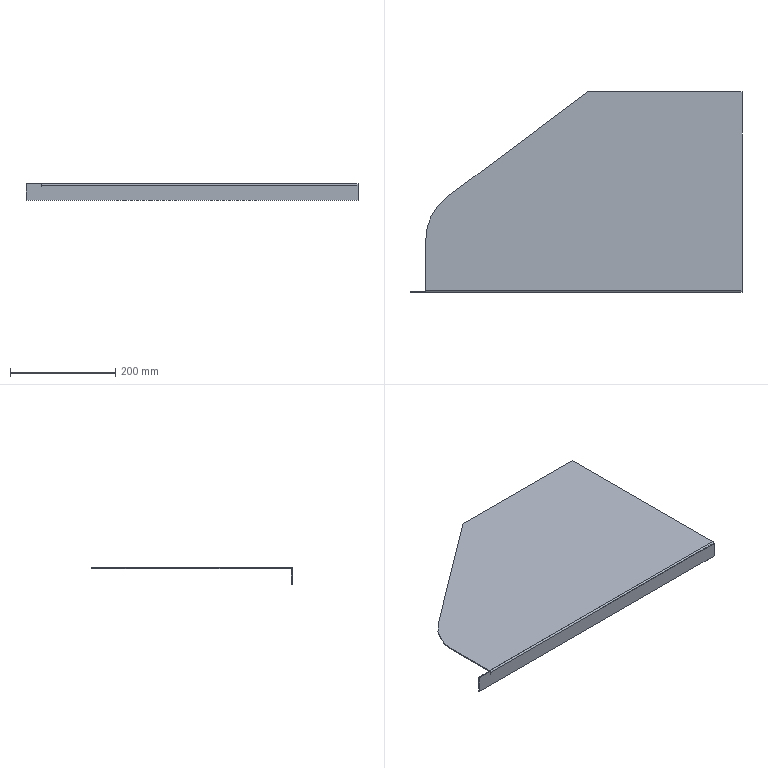Part | SolidWorks | features ICE 5, Split 4, DeleteBody 3, Extrusion 1, FlatPattern 1, SheetMetal 1, Shell 1, SolidToSheetMetal 1 | 1 solid | 20 faces | box 630 x 380 x 32 mm | volume 421618 mm3 | plane 17 | cylinder 3 | commonest cylinder face diameters 2 x1 6 x1 200 x1
STEP:
#1=CARTESIAN_POINT('',(-1100.,3.,-298.));
#2=VERTEX_POINT('',#1);
#3=CARTESIAN_POINT('',(-1100.,3.,-300.));
#4=VERTEX_POINT('',#3);
#5=CARTESIAN_POINT('',(-1100.,3.,-300.));
#6=DIRECTION('',(0.,0.,-1.));
#7=VECTOR('',#6,1000.);
#8=LINE('',#5,#7);
#9=EDGE_CURVE('',#2,#4,#8,.T.);
#10=ORIENTED_EDGE('',*,*,#9,.F.);
#11=CARTESIAN_POINT('',(-1100.,100.,-298.));
#12=VERTEX_POINT('',#11);
#13=CARTESIAN_POINT('',(-1100.,100.,-298.));
#14=DIRECTION('',(0.,1.,0.));
#15=VECTOR('',#14,1000.);
#16=LINE('',#13,#15);
#17=EDGE_CURVE('',#2,#12,#16,.T.);
#18=ORIENTED_EDGE('',*,*,#17,.T.);
#19=CARTESIAN_POINT('',(-1100.,100.,-300.));
#20=VERTEX_POINT('',#19);
#21=CARTESIAN_POINT('',(-1100.,100.,-300.));
#22=DIRECTION('',(0.,0.,-1.));
#23=VECTOR('',#22,1000.);
#24=LINE('',#21,#23);
#25=EDGE_CURVE('',#12,#20,#24,.T.);
#26=ORIENTED_EDGE('',*,*,#25,.T.);
#27=CARTESIAN_POINT('',(-1100.,100.,-300.));
#28=DIRECTION('',(0.,1.,0.));
#29=VECTOR('',#28,1000.);
#30=LINE('',#27,#29);
#31=EDGE_CURVE('',#4,#20,#30,.T.);
#32=ORIENTED_EDGE('',*,*,#31,.F.);
#33=EDGE_LOOP('',(#10,#18,#26,#32));
#34=FACE_OUTER_BOUND('',#33,.T.);
#35=CARTESIAN_POINT('',(-1100.,100.,-300.));
#36=DIRECTION('',(-1.,0.,0.));
#37=DIRECTION('',(0.,1.,0.));
#38=AXIS2_PLACEMENT_3D('',#35,#36,#37);
#39=PLANE('',#38);
#40=ADVANCED_FACE('',(#34),#39,.T.);
#41=ORIENTED_EDGE('',*,*,#25,.F.);
#42=CARTESIAN_POINT('',(-1060.,180.,-298.));
#43=VERTEX_POINT('',#42);
#44=CARTESIAN_POINT('',(-1000.,100.,-298.));
#45=DIRECTION('',(0.,0.,-1.));
#46=DIRECTION('',(-1.,0.,0.));
#47=AXIS2_PLACEMENT_3D('',#44,#45,#46);
#48=CIRCLE('',#47,100.);
#49=EDGE_CURVE('',#12,#43,#48,.T.);
#50=ORIENTED_EDGE('',*,*,#49,.T.);
#51=CARTESIAN_POINT('',(-1060.,180.,-300.));
#52=VERTEX_POINT('',#51);
#53=CARTESIAN_POINT('',(-1060.,180.,-300.));
#54=DIRECTION('',(0.,0.,-1.));
#55=VECTOR('',#54,1000.);
#56=LINE('',#53,#55);
#57=EDGE_CURVE('',#43,#52,#56,.T.);
#58=ORIENTED_EDGE('',*,*,#57,.T.);
#59=CARTESIAN_POINT('',(-1000.,100.,-300.));
#60=DIRECTION('',(0.,0.,-1.));
#61=DIRECTION('',(-1.,0.,0.));
#62=AXIS2_PLACEMENT_3D('',#59,#60,#61);
#63=CIRCLE('',#62,100.);
#64=EDGE_CURVE('',#20,#52,#63,.T.);
#65=ORIENTED_EDGE('',*,*,#64,.F.);
#66=EDGE_LOOP('',(#41,#50,#58,#65));
#67=FACE_OUTER_BOUND('',#66,.T.);
#68=CARTESIAN_POINT('',(-1000.,100.,-300.));
#69=DIRECTION('',(0.,0.,-1.));
#70=DIRECTION('',(-1.,0.,0.));
#71=AXIS2_PLACEMENT_3D('',#68,#69,#70);
#72=CYLINDRICAL_SURFACE('',#71,100.);
#73=ADVANCED_FACE('',(#67),#72,.T.);
#74=ORIENTED_EDGE('',*,*,#57,.F.);
#75=CARTESIAN_POINT('',(-793.333,380.,-298.));
#76=VERTEX_POINT('',#75);
#77=CARTESIAN_POINT('',(-793.333,380.,-298.));
#78=DIRECTION('',(0.8,0.6,0.));
#79=VECTOR('',#78,1000.);
#80=LINE('',#77,#79);
#81=EDGE_CURVE('',#43,#76,#80,.T.);
#82=ORIENTED_EDGE('',*,*,#81,.T.);
#83=CARTESIAN_POINT('',(-793.333,380.,-300.));
#84=VERTEX_POINT('',#83);
#85=CARTESIAN_POINT('',(-793.333,380.,-300.));
#86=DIRECTION('',(0.,0.,-1.));
#87=VECTOR('',#86,1000.);
#88=LINE('',#85,#87);
#89=EDGE_CURVE('',#76,#84,#88,.T.);
#90=ORIENTED_EDGE('',*,*,#89,.T.);
#91=CARTESIAN_POINT('',(-793.333,380.,-300.));
#92=DIRECTION('',(0.8,0.6,0.));
#93=VECTOR('',#92,1000.);
#94=LINE('',#91,#93);
#95=EDGE_CURVE('',#52,#84,#94,.T.);
#96=ORIENTED_EDGE('',*,*,#95,.F.);
#97=EDGE_LOOP('',(#74,#82,#90,#96));
#98=FACE_OUTER_BOUND('',#97,.T.);
#99=CARTESIAN_POINT('',(-793.333,380.,-300.));
#100=DIRECTION('',(-0.6,0.8,0.));
#101=DIRECTION('',(0.8,0.6,0.));
#102=AXIS2_PLACEMENT_3D('',#99,#100,#101);
#103=PLANE('',#102);
#104=ADVANCED_FACE('',(#98),#103,.T.);
#105=ORIENTED_EDGE('',*,*,#89,.F.);
#106=CARTESIAN_POINT('',(-500.,380.,-298.));
#107=VERTEX_POINT('',#106);
#108=CARTESIAN_POINT('',(-1000.,380.,-298.));
#109=DIRECTION('',(1.,0.,0.));
#110=VECTOR('',#109,1000.);
#111=LINE('',#108,#110);
#112=EDGE_CURVE('',#76,#107,#111,.T.);
#113=ORIENTED_EDGE('',*,*,#112,.T.);
#114=CARTESIAN_POINT('',(-500.,380.,-300.));
#115=VERTEX_POINT('',#114);
#116=CARTESIAN_POINT('',(-500.,380.,-300.));
#117=DIRECTION('',(0.,0.,-1.));
#118=VECTOR('',#117,1000.);
#119=LINE('',#116,#118);
#120=EDGE_CURVE('',#107,#115,#119,.T.);
#121=ORIENTED_EDGE('',*,*,#120,.T.);
#122=CARTESIAN_POINT('',(-793.333,380.,-300.));
#123=DIRECTION('',(1.,0.,0.));
#124=VECTOR('',#123,1000.);
#125=LINE('',#122,#124);
#126=EDGE_CURVE('',#84,#115,#125,.T.);
#127=ORIENTED_EDGE('',*,*,#126,.F.);
#128=EDGE_LOOP('',(#105,#113,#121,#127));
#129=FACE_OUTER_BOUND('',#128,.T.);
#130=CARTESIAN_POINT('',(-793.333,380.,-300.));
#131=DIRECTION('',(0.,1.,0.));
#132=DIRECTION('',(1.,0.,0.));
#133=AXIS2_PLACEMENT_3D('',#130,#131,#132);
#134=PLANE('',#133);
#135=ADVANCED_FACE('',(#129),#134,.T.);
#136=ORIENTED_EDGE('',*,*,#120,.F.);
#137=CARTESIAN_POINT('',(-500.,3.,-298.));
#138=VERTEX_POINT('',#137);
#139=CARTESIAN_POINT('',(-500.,100.,-298.));
#140=DIRECTION('',(0.,-1.,0.));
#141=VECTOR('',#140,1000.);
#142=LINE('',#139,#141);
#143=EDGE_CURVE('',#107,#138,#142,.T.);
#144=ORIENTED_EDGE('',*,*,#143,.T.);
#145=CARTESIAN_POINT('',(-500.,3.,-300.));
#146=VERTEX_POINT('',#145);
#147=CARTESIAN_POINT('',(-500.,3.,-300.));
#148=DIRECTION('',(0.,0.,-1.));
#149=VECTOR('',#148,1000.);
#150=LINE('',#147,#149);
#151=EDGE_CURVE('',#138,#146,#150,.T.);
#152=ORIENTED_EDGE('',*,*,#151,.T.);
#153=CARTESIAN_POINT('',(-500.,380.,-300.));
#154=DIRECTION('',(0.,-1.,0.));
#155=VECTOR('',#154,1000.);
#156=LINE('',#153,#155);
#157=EDGE_CURVE('',#115,#146,#156,.T.);
#158=ORIENTED_EDGE('',*,*,#157,.F.);
#159=EDGE_LOOP('',(#136,#144,#152,#158));
#160=FACE_OUTER_BOUND('',#159,.T.);
#161=CARTESIAN_POINT('',(-500.,380.,-300.));
#162=DIRECTION('',(1.,0.,0.));
#163=DIRECTION('',(0.,-1.,0.));
#164=AXIS2_PLACEMENT_3D('',#161,#162,#163);
#165=PLANE('',#164);
#166=ADVANCED_FACE('',(#160),#165,.T.);
#167=ORIENTED_EDGE('',*,*,#151,.F.);
#168=CARTESIAN_POINT('',(-500.,0.,-301.));
#169=VERTEX_POINT('',#168);
#170=CARTESIAN_POINT('',(-500.,3.,-301.));
#171=DIRECTION('',(1.,0.,0.));
#172=DIRECTION('',(0.,0.,-1.));
#173=AXIS2_PLACEMENT_3D('',#170,#171,#172);
#174=CIRCLE('',#173,3.);
#175=EDGE_CURVE('',#138,#169,#174,.T.);
#176=ORIENTED_EDGE('',*,*,#175,.T.);
#177=CARTESIAN_POINT('',(-500.,2.,-301.));
#178=VERTEX_POINT('',#177);
#179=CARTESIAN_POINT('',(-500.,2.,-301.));
#180=DIRECTION('',(0.,1.,0.));
#181=VECTOR('',#180,1000.);
#182=LINE('',#179,#181);
#183=EDGE_CURVE('',#169,#178,#182,.T.);
#184=ORIENTED_EDGE('',*,*,#183,.T.);
#185=CARTESIAN_POINT('',(-500.,3.,-301.));
#186=DIRECTION('',(1.,0.,0.));
#187=DIRECTION('',(0.,0.,1.));
#188=AXIS2_PLACEMENT_3D('',#185,#186,#187);
#189=CIRCLE('',#188,1.);
#190=EDGE_CURVE('',#146,#178,#189,.T.);
#191=ORIENTED_EDGE('',*,*,#190,.F.);
#192=EDGE_LOOP('',(#167,#176,#184,#191));
#193=FACE_OUTER_BOUND('',#192,.T.);
#194=CARTESIAN_POINT('',(-500.,3.,-301.));
#195=DIRECTION('',(1.,0.,0.));
#196=DIRECTION('',(0.,0.,-1.));
#197=AXIS2_PLACEMENT_3D('',#194,#195,#196);
#198=PLANE('',#197);
#199=ADVANCED_FACE('',(#193),#198,.T.);
#200=ORIENTED_EDGE('',*,*,#183,.F.);
#201=CARTESIAN_POINT('',(-500.,0.,-330.));
#202=VERTEX_POINT('',#201);
#203=CARTESIAN_POINT('',(-500.,0.,0.));
#204=DIRECTION('',(0.,0.,-1.));
#205=VECTOR('',#204,1000.);
#206=LINE('',#203,#205);
#207=EDGE_CURVE('',#169,#202,#206,.T.);
#208=ORIENTED_EDGE('',*,*,#207,.T.);
#209=CARTESIAN_POINT('',(-500.,2.,-330.));
#210=VERTEX_POINT('',#209);
#211=CARTESIAN_POINT('',(-500.,2.,-330.));
#212=DIRECTION('',(0.,1.,0.));
#213=VECTOR('',#212,1000.);
#214=LINE('',#211,#213);
#215=EDGE_CURVE('',#202,#210,#214,.T.);
#216=ORIENTED_EDGE('',*,*,#215,.T.);
#217=CARTESIAN_POINT('',(-500.,2.,0.));
#218=DIRECTION('',(0.,0.,-1.));
#219=VECTOR('',#218,1000.);
#220=LINE('',#217,#219);
#221=EDGE_CURVE('',#178,#210,#220,.T.);
#222=ORIENTED_EDGE('',*,*,#221,.F.);
#223=EDGE_LOOP('',(#200,#208,#216,#222));
#224=FACE_OUTER_BOUND('',#223,.T.);
#225=CARTESIAN_POINT('',(-500.,2.,0.));
#226=DIRECTION('',(1.,0.,0.));
#227=DIRECTION('',(0.,0.,-1.));
#228=AXIS2_PLACEMENT_3D('',#225,#226,#227);
#229=PLANE('',#228);
#230=ADVANCED_FACE('',(#224),#229,.T.);
#231=ORIENTED_EDGE('',*,*,#215,.F.);
#232=CARTESIAN_POINT('',(-1130.,0.,-330.));
#233=VERTEX_POINT('',#232);
#234=CARTESIAN_POINT('',(0.,0.,-330.));
#235=DIRECTION('',(1.,0.,0.));
#236=VECTOR('',#235,1000.);
#237=LINE('',#234,#236);
#238=EDGE_CURVE('',#233,#202,#237,.T.);
#239=ORIENTED_EDGE('',*,*,#238,.F.);
#240=CARTESIAN_POINT('',(-1130.,2.,-330.));
#241=VERTEX_POINT('',#240);
#242=CARTESIAN_POINT('',(-1130.,2.,-330.));
#243=DIRECTION('',(0.,1.,0.));
#244=VECTOR('',#243,1000.);
#245=LINE('',#242,#244);
#246=EDGE_CURVE('',#233,#241,#245,.T.);
#247=ORIENTED_EDGE('',*,*,#246,.T.);
#248=CARTESIAN_POINT('',(-1130.,2.,-330.));
#249=DIRECTION('',(1.,0.,0.));
#250=VECTOR('',#249,1000.);
#251=LINE('',#248,#250);
#252=EDGE_CURVE('',#241,#210,#251,.T.);
#253=ORIENTED_EDGE('',*,*,#252,.T.);
#254=EDGE_LOOP('',(#231,#239,#247,#253));
#255=FACE_OUTER_BOUND('',#254,.T.);
#256=CARTESIAN_POINT('',(-1130.,2.,-330.));
#257=DIRECTION('',(0.,0.,1.));
#258=DIRECTION('',(1.,0.,0.));
#259=AXIS2_PLACEMENT_3D('',#256,#257,#258);
#260=PLANE('',#259);
#261=ADVANCED_FACE('',(#255),#260,.F.);
#262=ORIENTED_EDGE('',*,*,#246,.F.);
#263=CARTESIAN_POINT('',(-1130.,0.,-298.));
#264=VERTEX_POINT('',#263);
#265=CARTESIAN_POINT('',(-1130.,0.,0.));
#266=DIRECTION('',(0.,0.,-1.));
#267=VECTOR('',#266,1000.);
#268=LINE('',#265,#267);
#269=EDGE_CURVE('',#264,#233,#268,.T.);
#270=ORIENTED_EDGE('',*,*,#269,.F.);
#271=CARTESIAN_POINT('',(-1130.,2.,-298.));
#272=VERTEX_POINT('',#271);
#273=CARTESIAN_POINT('',(-1130.,2.,-298.));
#274=DIRECTION('',(0.,1.,0.));
#275=VECTOR('',#274,1000.);
#276=LINE('',#273,#275);
#277=EDGE_CURVE('',#264,#272,#276,.T.);
#278=ORIENTED_EDGE('',*,*,#277,.T.);
#279=CARTESIAN_POINT('',(-1130.,2.,0.));
#280=DIRECTION('',(0.,0.,-1.));
#281=VECTOR('',#280,1000.);
#282=LINE('',#279,#281);
#283=EDGE_CURVE('',#272,#241,#282,.T.);
#284=ORIENTED_EDGE('',*,*,#283,.T.);
#285=EDGE_LOOP('',(#262,#270,#278,#284));
#286=FACE_OUTER_BOUND('',#285,.T.);
#287=CARTESIAN_POINT('',(-1130.,2.,0.));
#288=DIRECTION('',(1.,0.,0.));
#289=DIRECTION('',(0.,0.,-1.));
#290=AXIS2_PLACEMENT_3D('',#287,#288,#289);
#291=PLANE('',#290);
#292=ADVANCED_FACE('',(#286),#291,.F.);
#293=ORIENTED_EDGE('',*,*,#277,.F.);
#294=CARTESIAN_POINT('',(-1101.,0.,-298.));
#295=VERTEX_POINT('',#294);
#296=CARTESIAN_POINT('',(0.,0.,-298.));
#297=DIRECTION('',(1.,0.,0.));
#298=VECTOR('',#297,1000.);
#299=LINE('',#296,#298);
#300=EDGE_CURVE('',#264,#295,#299,.T.);
#301=ORIENTED_EDGE('',*,*,#300,.T.);
#302=CARTESIAN_POINT('',(-1101.,2.,-298.));
#303=VERTEX_POINT('',#302);
#304=CARTESIAN_POINT('',(-1101.,2.,-298.));
#305=DIRECTION('',(0.,1.,0.));
#306=VECTOR('',#305,1000.);
#307=LINE('',#304,#306);
#308=EDGE_CURVE('',#295,#303,#307,.T.);
#309=ORIENTED_EDGE('',*,*,#308,.T.);
#310=CARTESIAN_POINT('',(0.,2.,-298.));
#311=DIRECTION('',(1.,0.,0.));
#312=VECTOR('',#311,1000.);
#313=LINE('',#310,#312);
#314=EDGE_CURVE('',#272,#303,#313,.T.);
#315=ORIENTED_EDGE('',*,*,#314,.F.);
#316=EDGE_LOOP('',(#293,#301,#309,#315));
#317=FACE_OUTER_BOUND('',#316,.T.);
#318=CARTESIAN_POINT('',(0.,2.,-298.));
#319=DIRECTION('',(0.,0.,1.));
#320=DIRECTION('',(1.,0.,0.));
#321=AXIS2_PLACEMENT_3D('',#318,#319,#320);
#322=PLANE('',#321);
#323=ADVANCED_FACE('',(#317),#322,.T.);
#324=ORIENTED_EDGE('',*,*,#308,.F.);
#325=CARTESIAN_POINT('',(-1101.,0.,-304.));
#326=VERTEX_POINT('',#325);
#327=CARTESIAN_POINT('',(-1101.,0.,0.));
#328=DIRECTION('',(0.,0.,1.));
#329=VECTOR('',#328,1000.);
#330=LINE('',#327,#329);
#331=EDGE_CURVE('',#326,#295,#330,.T.);
#332=ORIENTED_EDGE('',*,*,#331,.F.);
#333=CARTESIAN_POINT('',(-1101.,2.,-304.));
#334=VERTEX_POINT('',#333);
#335=CARTESIAN_POINT('',(-1101.,2.,-304.));
#336=DIRECTION('',(0.,1.,0.));
#337=VECTOR('',#336,1000.);
#338=LINE('',#335,#337);
#339=EDGE_CURVE('',#326,#334,#338,.T.);
#340=ORIENTED_EDGE('',*,*,#339,.T.);
#341=CARTESIAN_POINT('',(-1101.,2.,0.));
#342=DIRECTION('',(0.,0.,1.));
#343=VECTOR('',#342,1000.);
#344=LINE('',#341,#343);
#345=EDGE_CURVE('',#334,#303,#344,.T.);
#346=ORIENTED_EDGE('',*,*,#345,.T.);
#347=EDGE_LOOP('',(#324,#332,#340,#346));
#348=FACE_OUTER_BOUND('',#347,.T.);
#349=CARTESIAN_POINT('',(-1101.,2.,0.));
#350=DIRECTION('',(-1.,0.,0.));
#351=DIRECTION('',(0.,0.,1.));
#352=AXIS2_PLACEMENT_3D('',#349,#350,#351);
#353=PLANE('',#352);
#354=ADVANCED_FACE('',(#348),#353,.F.);
#355=ORIENTED_EDGE('',*,*,#339,.F.);
#356=CARTESIAN_POINT('',(-1100.,0.,-304.));
#357=VERTEX_POINT('',#356);
#358=CARTESIAN_POINT('',(0.,0.,-304.));
#359=DIRECTION('',(-1.,0.,0.));
#360=VECTOR('',#359,1000.);
#361=LINE('',#358,#360);
#362=EDGE_CURVE('',#357,#326,#361,.T.);
#363=ORIENTED_EDGE('',*,*,#362,.F.);
#364=CARTESIAN_POINT('',(-1100.,2.,-304.));
#365=VERTEX_POINT('',#364);
#366=CARTESIAN_POINT('',(-1100.,2.,-304.));
#367=DIRECTION('',(0.,1.,0.));
#368=VECTOR('',#367,1000.);
#369=LINE('',#366,#368);
#370=EDGE_CURVE('',#357,#365,#369,.T.);
#371=ORIENTED_EDGE('',*,*,#370,.T.);
#372=CARTESIAN_POINT('',(0.,2.,-304.));
#373=DIRECTION('',(-1.,0.,0.));
#374=VECTOR('',#373,1000.);
#375=LINE('',#372,#374);
#376=EDGE_CURVE('',#365,#334,#375,.T.);
#377=ORIENTED_EDGE('',*,*,#376,.T.);
#378=EDGE_LOOP('',(#355,#363,#371,#377));
#379=FACE_OUTER_BOUND('',#378,.T.);
#380=CARTESIAN_POINT('',(0.,2.,-304.));
#381=DIRECTION('',(0.,0.,-1.));
#382=DIRECTION('',(-1.,0.,0.));
#383=AXIS2_PLACEMENT_3D('',#380,#381,#382);
#384=PLANE('',#383);
#385=ADVANCED_FACE('',(#379),#384,.F.);
#386=ORIENTED_EDGE('',*,*,#370,.F.);
#387=CARTESIAN_POINT('',(-1100.,0.,-301.));
#388=VERTEX_POINT('',#387);
#389=CARTESIAN_POINT('',(-1100.,0.,0.));
#390=DIRECTION('',(0.,0.,-1.));
#391=VECTOR('',#390,1000.);
#392=LINE('',#389,#391);
#393=EDGE_CURVE('',#388,#357,#392,.T.);
#394=ORIENTED_EDGE('',*,*,#393,.F.);
#395=CARTESIAN_POINT('',(-1100.,2.,-301.));
#396=VERTEX_POINT('',#395);
#397=CARTESIAN_POINT('',(-1100.,2.,-301.));
#398=DIRECTION('',(0.,1.,0.));
#399=VECTOR('',#398,1000.);
#400=LINE('',#397,#399);
#401=EDGE_CURVE('',#388,#396,#400,.T.);
#402=ORIENTED_EDGE('',*,*,#401,.T.);
#403=CARTESIAN_POINT('',(-1100.,2.,0.));
#404=DIRECTION('',(0.,0.,-1.));
#405=VECTOR('',#404,1000.);
#406=LINE('',#403,#405);
#407=EDGE_CURVE('',#396,#365,#406,.T.);
#408=ORIENTED_EDGE('',*,*,#407,.T.);
#409=EDGE_LOOP('',(#386,#394,#402,#408));
#410=FACE_OUTER_BOUND('',#409,.T.);
#411=CARTESIAN_POINT('',(-1100.,2.,0.));
#412=DIRECTION('',(1.,0.,0.));
#413=DIRECTION('',(0.,0.,-1.));
#414=AXIS2_PLACEMENT_3D('',#411,#412,#413);
#415=PLANE('',#414);
#416=ADVANCED_FACE('',(#410),#415,.F.);
#417=CARTESIAN_POINT('',(-1100.,3.,-301.));
#418=DIRECTION('',(-1.,0.,0.));
#419=DIRECTION('',(0.,0.,-1.));
#420=AXIS2_PLACEMENT_3D('',#417,#418,#419);
#421=CIRCLE('',#420,3.);
#422=EDGE_CURVE('',#388,#2,#421,.T.);
#423=ORIENTED_EDGE('',*,*,#422,.T.);
#424=ORIENTED_EDGE('',*,*,#9,.T.);
#425=CARTESIAN_POINT('',(-1100.,3.,-301.));
#426=DIRECTION('',(-1.,0.,0.));
#427=DIRECTION('',(0.,0.,1.));
#428=AXIS2_PLACEMENT_3D('',#425,#426,#427);
#429=CIRCLE('',#428,1.);
#430=EDGE_CURVE('',#396,#4,#429,.T.);
#431=ORIENTED_EDGE('',*,*,#430,.F.);
#432=ORIENTED_EDGE('',*,*,#401,.F.);
#433=EDGE_LOOP('',(#423,#424,#431,#432));
#434=FACE_OUTER_BOUND('',#433,.T.);
#435=CARTESIAN_POINT('',(-1100.,3.,-301.));
#436=DIRECTION('',(1.,0.,0.));
#437=DIRECTION('',(0.,0.,-1.));
#438=AXIS2_PLACEMENT_3D('',#435,#436,#437);
#439=PLANE('',#438);
#440=ADVANCED_FACE('',(#434),#439,.F.);
#441=ORIENTED_EDGE('',*,*,#407,.F.);
#442=CARTESIAN_POINT('',(-500.,2.,-301.));
#443=DIRECTION('',(1.,0.,0.));
#444=VECTOR('',#443,1000.);
#445=LINE('',#442,#444);
#446=EDGE_CURVE('',#396,#178,#445,.T.);
#447=ORIENTED_EDGE('',*,*,#446,.T.);
#448=ORIENTED_EDGE('',*,*,#221,.T.);
#449=ORIENTED_EDGE('',*,*,#252,.F.);
#450=ORIENTED_EDGE('',*,*,#283,.F.);
#451=ORIENTED_EDGE('',*,*,#314,.T.);
#452=ORIENTED_EDGE('',*,*,#345,.F.);
#453=ORIENTED_EDGE('',*,*,#376,.F.);
#454=EDGE_LOOP('',(#441,#447,#448,#449,#450,#451,#452,#453));
#455=FACE_OUTER_BOUND('',#454,.T.);
#456=CARTESIAN_POINT('',(0.,2.,0.));
#457=DIRECTION('',(0.,1.,0.));
#458=DIRECTION('',(0.,0.,1.));
#459=AXIS2_PLACEMENT_3D('',#456,#457,#458);
#460=PLANE('',#459);
#461=ADVANCED_FACE('',(#455),#460,.T.);
#462=ORIENTED_EDGE('',*,*,#157,.T.);
#463=CARTESIAN_POINT('',(-1100.,3.,-300.));
#464=DIRECTION('',(-1.,0.,0.));
#465=VECTOR('',#464,1000.);
#466=LINE('',#463,#465);
#467=EDGE_CURVE('',#146,#4,#466,.T.);
#468=ORIENTED_EDGE('',*,*,#467,.T.);
#469=ORIENTED_EDGE('',*,*,#31,.T.);
#470=ORIENTED_EDGE('',*,*,#64,.T.);
#471=ORIENTED_EDGE('',*,*,#95,.T.);
#472=ORIENTED_EDGE('',*,*,#126,.T.);
#473=EDGE_LOOP('',(#462,#468,#469,#470,#471,#472));
#474=FACE_OUTER_BOUND('',#473,.T.);
#475=CARTESIAN_POINT('',(-1000.,100.,-300.));
#476=DIRECTION('',(0.,0.,-1.));
#477=DIRECTION('',(-1.,0.,0.));
#478=AXIS2_PLACEMENT_3D('',#475,#476,#477);
#479=PLANE('',#478);
#480=ADVANCED_FACE('',(#474),#479,.T.);
#481=ORIENTED_EDGE('',*,*,#190,.T.);
#482=ORIENTED_EDGE('',*,*,#446,.F.);
#483=ORIENTED_EDGE('',*,*,#430,.T.);
#484=ORIENTED_EDGE('',*,*,#467,.F.);
#485=EDGE_LOOP('',(#481,#482,#483,#484));
#486=FACE_OUTER_BOUND('',#485,.T.);
#487=CARTESIAN_POINT('',(-1000.,3.,-301.));
#488=DIRECTION('',(1.,0.,0.));
#489=DIRECTION('',(0.,0.,-1.));
#490=AXIS2_PLACEMENT_3D('',#487,#488,#489);
#491=CYLINDRICAL_SURFACE('',#490,1.);
#492=ADVANCED_FACE('',(#486),#491,.F.);
#493=ORIENTED_EDGE('',*,*,#393,.T.);
#494=ORIENTED_EDGE('',*,*,#362,.T.);
#495=ORIENTED_EDGE('',*,*,#331,.T.);
#496=ORIENTED_EDGE('',*,*,#300,.F.);
#497=ORIENTED_EDGE('',*,*,#269,.T.);
#498=ORIENTED_EDGE('',*,*,#238,.T.);
#499=ORIENTED_EDGE('',*,*,#207,.F.);
#500=CARTESIAN_POINT('',(0.,0.,-301.));
#501=DIRECTION('',(1.,0.,0.));
#502=VECTOR('',#501,1000.);
#503=LINE('',#500,#502);
#504=EDGE_CURVE('',#388,#169,#503,.T.);
#505=ORIENTED_EDGE('',*,*,#504,.F.);
#506=EDGE_LOOP('',(#493,#494,#495,#496,#497,#498,#499,#505));
#507=FACE_OUTER_BOUND('',#506,.T.);
#508=CARTESIAN_POINT('',(0.,0.,0.));
#509=DIRECTION('',(0.,1.,0.));
#510=DIRECTION('',(0.,0.,1.));
#511=AXIS2_PLACEMENT_3D('',#508,#509,#510);
#512=PLANE('',#511);
#513=ADVANCED_FACE('',(#507),#512,.F.);
#514=ORIENTED_EDGE('',*,*,#143,.F.);
#515=ORIENTED_EDGE('',*,*,#112,.F.);
#516=ORIENTED_EDGE('',*,*,#81,.F.);
#517=ORIENTED_EDGE('',*,*,#49,.F.);
#518=ORIENTED_EDGE('',*,*,#17,.F.);
#519=CARTESIAN_POINT('',(-1000.,3.,-298.));
#520=DIRECTION('',(-1.,0.,0.));
#521=VECTOR('',#520,1000.);
#522=LINE('',#519,#521);
#523=EDGE_CURVE('',#138,#2,#522,.T.);
#524=ORIENTED_EDGE('',*,*,#523,.F.);
#525=EDGE_LOOP('',(#514,#515,#516,#517,#518,#524));
#526=FACE_OUTER_BOUND('',#525,.T.);
#527=CARTESIAN_POINT('',(-1000.,100.,-298.));
#528=DIRECTION('',(0.,0.,-1.));
#529=DIRECTION('',(-1.,0.,0.));
#530=AXIS2_PLACEMENT_3D('',#527,#528,#529);
#531=PLANE('',#530);
#532=ADVANCED_FACE('',(#526),#531,.F.);
#533=ORIENTED_EDGE('',*,*,#175,.F.);
#534=ORIENTED_EDGE('',*,*,#523,.T.);
#535=ORIENTED_EDGE('',*,*,#422,.F.);
#536=ORIENTED_EDGE('',*,*,#504,.T.);
#537=EDGE_LOOP('',(#533,#534,#535,#536));
#538=FACE_OUTER_BOUND('',#537,.T.);
#539=CARTESIAN_POINT('',(-1000.,3.,-301.));
#540=DIRECTION('',(1.,0.,0.));
#541=DIRECTION('',(0.,0.,-1.));
#542=AXIS2_PLACEMENT_3D('',#539,#540,#541);
#543=CYLINDRICAL_SURFACE('',#542,3.);
#544=ADVANCED_FACE('',(#538),#543,.T.);
#545=CLOSED_SHELL('',(#40,#73,#104,#135,#166,#199,#230,#261,#292,#323,#354,#385,#416,#440,#461,#480,#492,#513,#532,#544));
#546=MANIFOLD_SOLID_BREP('',#545);
#547=CARTESIAN_POINT('',(0.,0.,0.));
#548=DIRECTION('',(0.,0.,1.));
#549=DIRECTION('',(1.,0.,0.));
#550=AXIS2_PLACEMENT_3D('',#547,#548,#549);
#551=(LENGTH_UNIT()NAMED_UNIT(*)SI_UNIT(.MILLI.,.METRE.));
#552=UNCERTAINTY_MEASURE_WITH_UNIT(LENGTH_MEASURE(0.00001),#551,'','');
#553=(NAMED_UNIT(*)PLANE_ANGLE_UNIT()SI_UNIT($,.RADIAN.));
#554=(NAMED_UNIT(*)SI_UNIT($,.STERADIAN.)SOLID_ANGLE_UNIT());
#555=(GEOMETRIC_REPRESENTATION_CONTEXT(3)GLOBAL_UNCERTAINTY_ASSIGNED_CONTEXT((#552))GLOBAL_UNIT_ASSIGNED_CONTEXT((#551,#553,#554))REPRESENTATION_CONTEXT('',''));
#556=ADVANCED_BREP_SHAPE_REPRESENTATION('',(#546,#550),#555);